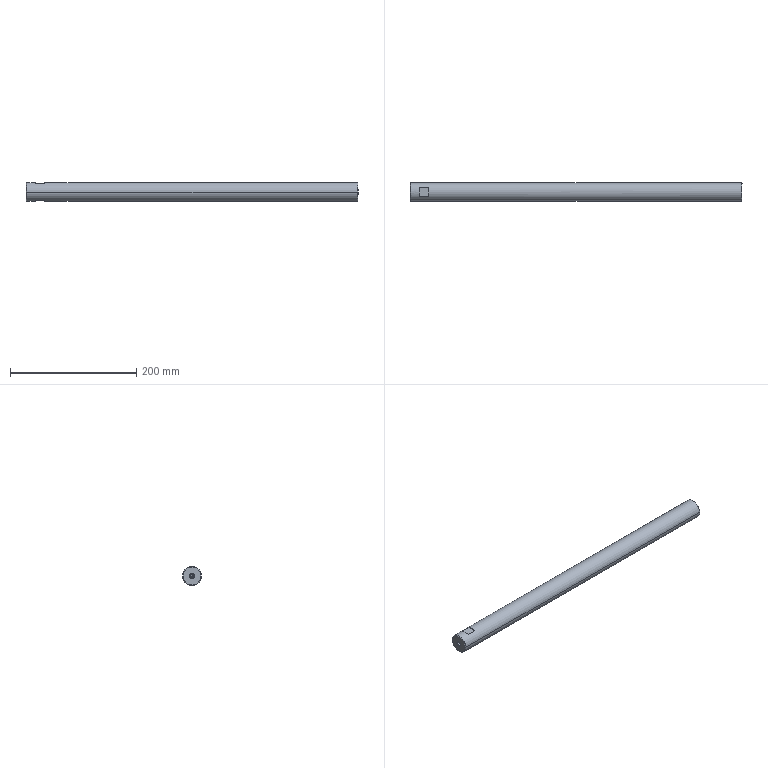Part | SolidWorks | features ICE 1, RevCut 1, Revolution 1 | 1 solid | 20 faces | box 525 x 30 x 30 mm | volume 369974 mm3 | cone 8 | plane 8 | cylinder 4 | commonest cylinder face diameters 6.647 x2 30 x2
STEP:
#1=CARTESIAN_POINT('',(19.519,0.,0.));
#2=VERTEX_POINT('',#1);
#3=CARTESIAN_POINT('',(17.6,-3.324,0.));
#4=VERTEX_POINT('',#3);
#5=CARTESIAN_POINT('',(19.519,0.,0.));
#6=DIRECTION('',(-0.5,-0.866,0.));
#7=VECTOR('',#6,1000.);
#8=LINE('',#5,#7);
#9=EDGE_CURVE('',#2,#4,#8,.T.);
#10=ORIENTED_EDGE('',*,*,#9,.F.);
#11=CARTESIAN_POINT('',(17.6,3.324,0.));
#12=VERTEX_POINT('',#11);
#13=CARTESIAN_POINT('',(19.519,0.,0.));
#14=DIRECTION('',(-0.5,0.866,0.));
#15=VECTOR('',#14,1000.);
#16=LINE('',#13,#15);
#17=EDGE_CURVE('',#2,#12,#16,.T.);
#18=ORIENTED_EDGE('',*,*,#17,.T.);
#19=CARTESIAN_POINT('',(17.6,0.,0.));
#20=DIRECTION('',(-1.,0.,0.));
#21=DIRECTION('',(0.,-1.,0.));
#22=AXIS2_PLACEMENT_3D('',#19,#20,#21);
#23=CIRCLE('',#22,3.324);
#24=EDGE_CURVE('',#12,#4,#23,.T.);
#25=ORIENTED_EDGE('',*,*,#24,.T.);
#26=EDGE_LOOP('',(#10,#18,#25));
#27=FACE_OUTER_BOUND('',#26,.T.);
#28=CARTESIAN_POINT('',(-980.481,0.,0.));
#29=DIRECTION('',(-1.,0.,0.));
#30=DIRECTION('',(0.,-1.,0.));
#31=AXIS2_PLACEMENT_3D('',#28,#29,#30);
#32=CONICAL_SURFACE('',#31,1732.051,1.047);
#33=ADVANCED_FACE('',(#27),#32,.F.);
#34=ORIENTED_EDGE('',*,*,#24,.F.);
#35=CARTESIAN_POINT('',(0.6765,3.324,0.));
#36=VERTEX_POINT('',#35);
#37=CARTESIAN_POINT('',(19.519,3.323,0.));
#38=DIRECTION('',(-1.,0.,0.));
#39=VECTOR('',#38,1000.);
#40=LINE('',#37,#39);
#41=EDGE_CURVE('',#12,#36,#40,.T.);
#42=ORIENTED_EDGE('',*,*,#41,.T.);
#43=CARTESIAN_POINT('',(0.6765,-3.324,0.));
#44=VERTEX_POINT('',#43);
#45=CARTESIAN_POINT('',(0.6765,0.,0.));
#46=DIRECTION('',(-1.,0.,0.));
#47=DIRECTION('',(0.,-1.,0.));
#48=AXIS2_PLACEMENT_3D('',#45,#46,#47);
#49=CIRCLE('',#48,3.324);
#50=EDGE_CURVE('',#36,#44,#49,.T.);
#51=ORIENTED_EDGE('',*,*,#50,.T.);
#52=CARTESIAN_POINT('',(19.519,-3.324,0.));
#53=DIRECTION('',(-1.,0.,0.));
#54=VECTOR('',#53,1000.);
#55=LINE('',#52,#54);
#56=EDGE_CURVE('',#4,#44,#55,.T.);
#57=ORIENTED_EDGE('',*,*,#56,.F.);
#58=EDGE_LOOP('',(#34,#42,#51,#57));
#59=FACE_OUTER_BOUND('',#58,.T.);
#60=CARTESIAN_POINT('',(19.519,0.,0.));
#61=DIRECTION('',(-1.,0.,0.));
#62=DIRECTION('',(0.,-1.,0.));
#63=AXIS2_PLACEMENT_3D('',#60,#61,#62);
#64=CYLINDRICAL_SURFACE('',#63,3.324);
#65=ADVANCED_FACE('',(#59),#64,.F.);
#66=ORIENTED_EDGE('',*,*,#50,.F.);
#67=CARTESIAN_POINT('',(0.,4.,0.));
#68=VERTEX_POINT('',#67);
#69=CARTESIAN_POINT('',(0.6765,3.324,0.));
#70=DIRECTION('',(-0.7071,0.7071,0.));
#71=VECTOR('',#70,1000.);
#72=LINE('',#69,#71);
#73=EDGE_CURVE('',#36,#68,#72,.T.);
#74=ORIENTED_EDGE('',*,*,#73,.T.);
#75=CARTESIAN_POINT('',(0.,-4.,0.));
#76=VERTEX_POINT('',#75);
#77=CARTESIAN_POINT('',(0.,0.,0.));
#78=DIRECTION('',(-1.,0.,0.));
#79=DIRECTION('',(0.,-1.,0.));
#80=AXIS2_PLACEMENT_3D('',#77,#78,#79);
#81=CIRCLE('',#80,4.);
#82=EDGE_CURVE('',#68,#76,#81,.T.);
#83=ORIENTED_EDGE('',*,*,#82,.T.);
#84=CARTESIAN_POINT('',(0.6765,-3.324,0.));
#85=DIRECTION('',(-0.7071,-0.7071,0.));
#86=VECTOR('',#85,1000.);
#87=LINE('',#84,#86);
#88=EDGE_CURVE('',#44,#76,#87,.T.);
#89=ORIENTED_EDGE('',*,*,#88,.F.);
#90=EDGE_LOOP('',(#66,#74,#83,#89));
#91=FACE_OUTER_BOUND('',#90,.T.);
#92=CARTESIAN_POINT('',(0.6765,0.,0.));
#93=DIRECTION('',(-1.,0.,0.));
#94=DIRECTION('',(0.,-1.,0.));
#95=AXIS2_PLACEMENT_3D('',#92,#93,#94);
#96=CONICAL_SURFACE('',#95,3.324,0.7854);
#97=ADVANCED_FACE('',(#91),#96,.F.);
#98=CARTESIAN_POINT('',(525.,-14.,0.));
#99=VERTEX_POINT('',#98);
#100=CARTESIAN_POINT('',(525.,14.,0.));
#101=VERTEX_POINT('',#100);
#102=CARTESIAN_POINT('',(525.,0.,0.));
#103=DIRECTION('',(-1.,0.,0.));
#104=DIRECTION('',(0.,-1.,0.));
#105=AXIS2_PLACEMENT_3D('',#102,#103,#104);
#106=CIRCLE('',#105,14.);
#107=EDGE_CURVE('',#99,#101,#106,.T.);
#108=ORIENTED_EDGE('',*,*,#107,.T.);
#109=CARTESIAN_POINT('',(524.,15.,0.));
#110=VERTEX_POINT('',#109);
#111=CARTESIAN_POINT('',(525.,14.,0.));
#112=DIRECTION('',(-0.7071,0.7071,0.));
#113=VECTOR('',#112,1000.);
#114=LINE('',#111,#113);
#115=EDGE_CURVE('',#101,#110,#114,.T.);
#116=ORIENTED_EDGE('',*,*,#115,.T.);
#117=CARTESIAN_POINT('',(524.,-15.,0.));
#118=VERTEX_POINT('',#117);
#119=CARTESIAN_POINT('',(524.,0.,0.));
#120=DIRECTION('',(-1.,0.,0.));
#121=DIRECTION('',(0.,-1.,0.));
#122=AXIS2_PLACEMENT_3D('',#119,#120,#121);
#123=CIRCLE('',#122,15.);
#124=EDGE_CURVE('',#118,#110,#123,.T.);
#125=ORIENTED_EDGE('',*,*,#124,.F.);
#126=CARTESIAN_POINT('',(525.,-14.,0.));
#127=DIRECTION('',(-0.7071,-0.7071,0.));
#128=VECTOR('',#127,1000.);
#129=LINE('',#126,#128);
#130=EDGE_CURVE('',#99,#118,#129,.T.);
#131=ORIENTED_EDGE('',*,*,#130,.F.);
#132=EDGE_LOOP('',(#108,#116,#125,#131));
#133=FACE_OUTER_BOUND('',#132,.T.);
#134=CARTESIAN_POINT('',(525.,0.,0.));
#135=DIRECTION('',(-1.,0.,0.));
#136=DIRECTION('',(0.,-1.,0.));
#137=AXIS2_PLACEMENT_3D('',#134,#135,#136);
#138=CONICAL_SURFACE('',#137,14.,0.7854);
#139=ADVANCED_FACE('',(#133),#138,.T.);
#140=CARTESIAN_POINT('',(30.,6.538,13.5));
#141=VERTEX_POINT('',#140);
#142=CARTESIAN_POINT('',(30.,-6.538,13.5));
#143=VERTEX_POINT('',#142);
#144=CARTESIAN_POINT('',(30.,0.,0.));
#145=DIRECTION('',(1.,0.,0.));
#146=DIRECTION('',(0.,0.,-1.));
#147=AXIS2_PLACEMENT_3D('',#144,#145,#146);
#148=CIRCLE('',#147,15.);
#149=EDGE_CURVE('',#141,#143,#148,.T.);
#150=ORIENTED_EDGE('',*,*,#149,.T.);
#151=CARTESIAN_POINT('',(15.,-6.538,13.5));
#152=VERTEX_POINT('',#151);
#153=CARTESIAN_POINT('',(525.,-6.538,13.5));
#154=DIRECTION('',(-1.,0.,0.));
#155=VECTOR('',#154,1000.);
#156=LINE('',#153,#155);
#157=EDGE_CURVE('',#143,#152,#156,.T.);
#158=ORIENTED_EDGE('',*,*,#157,.T.);
#159=CARTESIAN_POINT('',(15.,6.538,13.5));
#160=VERTEX_POINT('',#159);
#161=CARTESIAN_POINT('',(15.,0.,0.));
#162=DIRECTION('',(1.,0.,0.));
#163=DIRECTION('',(0.,0.,-1.));
#164=AXIS2_PLACEMENT_3D('',#161,#162,#163);
#165=CIRCLE('',#164,15.);
#166=EDGE_CURVE('',#160,#152,#165,.T.);
#167=ORIENTED_EDGE('',*,*,#166,.F.);
#168=CARTESIAN_POINT('',(525.,6.538,13.5));
#169=DIRECTION('',(1.,0.,0.));
#170=VECTOR('',#169,1000.);
#171=LINE('',#168,#170);
#172=EDGE_CURVE('',#160,#141,#171,.T.);
#173=ORIENTED_EDGE('',*,*,#172,.T.);
#174=EDGE_LOOP('',(#150,#158,#167,#173));
#175=FACE_BOUND('',#174,.T.);
#176=ORIENTED_EDGE('',*,*,#124,.T.);
#177=CARTESIAN_POINT('',(1.,15.,0.));
#178=VERTEX_POINT('',#177);
#179=CARTESIAN_POINT('',(525.,15.,0.));
#180=DIRECTION('',(-1.,0.,0.));
#181=VECTOR('',#180,1000.);
#182=LINE('',#179,#181);
#183=EDGE_CURVE('',#110,#178,#182,.T.);
#184=ORIENTED_EDGE('',*,*,#183,.T.);
#185=CARTESIAN_POINT('',(1.,-15.,0.));
#186=VERTEX_POINT('',#185);
#187=CARTESIAN_POINT('',(1.,0.,0.));
#188=DIRECTION('',(-1.,0.,0.));
#189=DIRECTION('',(0.,-1.,0.));
#190=AXIS2_PLACEMENT_3D('',#187,#188,#189);
#191=CIRCLE('',#190,15.);
#192=EDGE_CURVE('',#186,#178,#191,.T.);
#193=ORIENTED_EDGE('',*,*,#192,.F.);
#194=CARTESIAN_POINT('',(525.,-15.,0.));
#195=DIRECTION('',(-1.,0.,0.));
#196=VECTOR('',#195,1000.);
#197=LINE('',#194,#196);
#198=EDGE_CURVE('',#118,#186,#197,.T.);
#199=ORIENTED_EDGE('',*,*,#198,.F.);
#200=EDGE_LOOP('',(#176,#184,#193,#199));
#201=FACE_OUTER_BOUND('',#200,.T.);
#202=CARTESIAN_POINT('',(525.,0.,0.));
#203=DIRECTION('',(-1.,0.,0.));
#204=DIRECTION('',(0.,-1.,0.));
#205=AXIS2_PLACEMENT_3D('',#202,#203,#204);
#206=CYLINDRICAL_SURFACE('',#205,15.);
#207=ADVANCED_FACE('',(#175,#201),#206,.T.);
#208=CARTESIAN_POINT('',(0.,-14.,0.));
#209=VERTEX_POINT('',#208);
#210=CARTESIAN_POINT('',(0.,14.,0.));
#211=VERTEX_POINT('',#210);
#212=CARTESIAN_POINT('',(0.,0.,0.));
#213=DIRECTION('',(-1.,0.,0.));
#214=DIRECTION('',(0.,-1.,0.));
#215=AXIS2_PLACEMENT_3D('',#212,#213,#214);
#216=CIRCLE('',#215,14.);
#217=EDGE_CURVE('',#209,#211,#216,.T.);
#218=ORIENTED_EDGE('',*,*,#217,.F.);
#219=CARTESIAN_POINT('',(1.,-15.,0.));
#220=DIRECTION('',(0.7071,-0.7071,0.));
#221=VECTOR('',#220,1000.);
#222=LINE('',#219,#221);
#223=EDGE_CURVE('',#209,#186,#222,.T.);
#224=ORIENTED_EDGE('',*,*,#223,.T.);
#225=ORIENTED_EDGE('',*,*,#192,.T.);
#226=CARTESIAN_POINT('',(1.,15.,0.));
#227=DIRECTION('',(0.7071,0.7071,0.));
#228=VECTOR('',#227,1000.);
#229=LINE('',#226,#228);
#230=EDGE_CURVE('',#211,#178,#229,.T.);
#231=ORIENTED_EDGE('',*,*,#230,.F.);
#232=EDGE_LOOP('',(#218,#224,#225,#231));
#233=FACE_OUTER_BOUND('',#232,.T.);
#234=CARTESIAN_POINT('',(1.,0.,0.));
#235=DIRECTION('',(1.,0.,0.));
#236=DIRECTION('',(0.,1.,0.));
#237=AXIS2_PLACEMENT_3D('',#234,#235,#236);
#238=CONICAL_SURFACE('',#237,15.,0.7854);
#239=ADVANCED_FACE('',(#233),#238,.T.);
#240=CARTESIAN_POINT('',(0.,0.,0.));
#241=DIRECTION('',(-1.,0.,0.));
#242=DIRECTION('',(0.,-1.,0.));
#243=AXIS2_PLACEMENT_3D('',#240,#241,#242);
#244=CIRCLE('',#243,14.);
#245=EDGE_CURVE('',#211,#209,#244,.T.);
#246=ORIENTED_EDGE('',*,*,#245,.T.);
#247=ORIENTED_EDGE('',*,*,#217,.T.);
#248=EDGE_LOOP('',(#246,#247));
#249=FACE_OUTER_BOUND('',#248,.T.);
#250=CARTESIAN_POINT('',(0.,0.,0.));
#251=DIRECTION('',(-1.,0.,0.));
#252=DIRECTION('',(0.,-1.,0.));
#253=AXIS2_PLACEMENT_3D('',#250,#251,#252);
#254=CIRCLE('',#253,4.);
#255=EDGE_CURVE('',#76,#68,#254,.T.);
#256=ORIENTED_EDGE('',*,*,#255,.F.);
#257=ORIENTED_EDGE('',*,*,#82,.F.);
#258=EDGE_LOOP('',(#256,#257));
#259=FACE_BOUND('',#258,.T.);
#260=CARTESIAN_POINT('',(0.,0.,0.));
#261=DIRECTION('',(1.,0.,0.));
#262=DIRECTION('',(0.,1.,0.));
#263=AXIS2_PLACEMENT_3D('',#260,#261,#262);
#264=PLANE('',#263);
#265=ADVANCED_FACE('',(#249,#259),#264,.F.);
#266=ORIENTED_EDGE('',*,*,#223,.F.);
#267=ORIENTED_EDGE('',*,*,#245,.F.);
#268=ORIENTED_EDGE('',*,*,#230,.T.);
#269=CARTESIAN_POINT('',(1.,0.,0.));
#270=DIRECTION('',(-1.,0.,0.));
#271=DIRECTION('',(0.,-1.,0.));
#272=AXIS2_PLACEMENT_3D('',#269,#270,#271);
#273=CIRCLE('',#272,15.);
#274=EDGE_CURVE('',#178,#186,#273,.T.);
#275=ORIENTED_EDGE('',*,*,#274,.T.);
#276=EDGE_LOOP('',(#266,#267,#268,#275));
#277=FACE_OUTER_BOUND('',#276,.T.);
#278=CARTESIAN_POINT('',(1.,0.,0.));
#279=DIRECTION('',(1.,0.,0.));
#280=DIRECTION('',(0.,1.,0.));
#281=AXIS2_PLACEMENT_3D('',#278,#279,#280);
#282=CONICAL_SURFACE('',#281,15.,0.7854);
#283=ADVANCED_FACE('',(#277),#282,.T.);
#284=ORIENTED_EDGE('',*,*,#183,.F.);
#285=CARTESIAN_POINT('',(524.,0.,0.));
#286=DIRECTION('',(-1.,0.,0.));
#287=DIRECTION('',(0.,-1.,0.));
#288=AXIS2_PLACEMENT_3D('',#285,#286,#287);
#289=CIRCLE('',#288,15.);
#290=EDGE_CURVE('',#110,#118,#289,.T.);
#291=ORIENTED_EDGE('',*,*,#290,.T.);
#292=ORIENTED_EDGE('',*,*,#198,.T.);
#293=ORIENTED_EDGE('',*,*,#274,.F.);
#294=EDGE_LOOP('',(#284,#291,#292,#293));
#295=FACE_OUTER_BOUND('',#294,.T.);
#296=CARTESIAN_POINT('',(30.,-6.538,-13.5));
#297=VERTEX_POINT('',#296);
#298=CARTESIAN_POINT('',(30.,6.538,-13.5));
#299=VERTEX_POINT('',#298);
#300=CARTESIAN_POINT('',(30.,0.,0.));
#301=DIRECTION('',(1.,0.,0.));
#302=DIRECTION('',(0.,0.,-1.));
#303=AXIS2_PLACEMENT_3D('',#300,#301,#302);
#304=CIRCLE('',#303,15.);
#305=EDGE_CURVE('',#297,#299,#304,.T.);
#306=ORIENTED_EDGE('',*,*,#305,.T.);
#307=CARTESIAN_POINT('',(15.,6.538,-13.5));
#308=VERTEX_POINT('',#307);
#309=CARTESIAN_POINT('',(525.,6.538,-13.5));
#310=DIRECTION('',(-1.,0.,0.));
#311=VECTOR('',#310,1000.);
#312=LINE('',#309,#311);
#313=EDGE_CURVE('',#299,#308,#312,.T.);
#314=ORIENTED_EDGE('',*,*,#313,.T.);
#315=CARTESIAN_POINT('',(15.,-6.538,-13.5));
#316=VERTEX_POINT('',#315);
#317=CARTESIAN_POINT('',(15.,0.,0.));
#318=DIRECTION('',(1.,0.,0.));
#319=DIRECTION('',(0.,0.,-1.));
#320=AXIS2_PLACEMENT_3D('',#317,#318,#319);
#321=CIRCLE('',#320,15.);
#322=EDGE_CURVE('',#316,#308,#321,.T.);
#323=ORIENTED_EDGE('',*,*,#322,.F.);
#324=CARTESIAN_POINT('',(525.,-6.538,-13.5));
#325=DIRECTION('',(1.,0.,0.));
#326=VECTOR('',#325,1000.);
#327=LINE('',#324,#326);
#328=EDGE_CURVE('',#316,#297,#327,.T.);
#329=ORIENTED_EDGE('',*,*,#328,.T.);
#330=EDGE_LOOP('',(#306,#314,#323,#329));
#331=FACE_BOUND('',#330,.T.);
#332=CARTESIAN_POINT('',(525.,0.,0.));
#333=DIRECTION('',(-1.,0.,0.));
#334=DIRECTION('',(0.,-1.,0.));
#335=AXIS2_PLACEMENT_3D('',#332,#333,#334);
#336=CYLINDRICAL_SURFACE('',#335,15.);
#337=ADVANCED_FACE('',(#295,#331),#336,.T.);
#338=ORIENTED_EDGE('',*,*,#115,.F.);
#339=CARTESIAN_POINT('',(525.,0.,0.));
#340=DIRECTION('',(-1.,0.,0.));
#341=DIRECTION('',(0.,-1.,0.));
#342=AXIS2_PLACEMENT_3D('',#339,#340,#341);
#343=CIRCLE('',#342,14.);
#344=EDGE_CURVE('',#101,#99,#343,.T.);
#345=ORIENTED_EDGE('',*,*,#344,.T.);
#346=ORIENTED_EDGE('',*,*,#130,.T.);
#347=ORIENTED_EDGE('',*,*,#290,.F.);
#348=EDGE_LOOP('',(#338,#345,#346,#347));
#349=FACE_OUTER_BOUND('',#348,.T.);
#350=CARTESIAN_POINT('',(525.,0.,0.));
#351=DIRECTION('',(-1.,0.,0.));
#352=DIRECTION('',(0.,-1.,0.));
#353=AXIS2_PLACEMENT_3D('',#350,#351,#352);
#354=CONICAL_SURFACE('',#353,14.,0.7854);
#355=ADVANCED_FACE('',(#349),#354,.T.);
#356=ORIENTED_EDGE('',*,*,#107,.F.);
#357=ORIENTED_EDGE('',*,*,#344,.F.);
#358=EDGE_LOOP('',(#356,#357));
#359=FACE_OUTER_BOUND('',#358,.T.);
#360=CARTESIAN_POINT('',(525.,14.,0.));
#361=DIRECTION('',(-1.,0.,0.));
#362=DIRECTION('',(0.,-1.,0.));
#363=AXIS2_PLACEMENT_3D('',#360,#361,#362);
#364=PLANE('',#363);
#365=ADVANCED_FACE('',(#359),#364,.F.);
#366=ORIENTED_EDGE('',*,*,#73,.F.);
#367=CARTESIAN_POINT('',(0.6765,0.,0.));
#368=DIRECTION('',(-1.,0.,0.));
#369=DIRECTION('',(0.,-1.,0.));
#370=AXIS2_PLACEMENT_3D('',#367,#368,#369);
#371=CIRCLE('',#370,3.324);
#372=EDGE_CURVE('',#44,#36,#371,.T.);
#373=ORIENTED_EDGE('',*,*,#372,.F.);
#374=ORIENTED_EDGE('',*,*,#88,.T.);
#375=ORIENTED_EDGE('',*,*,#255,.T.);
#376=EDGE_LOOP('',(#366,#373,#374,#375));
#377=FACE_OUTER_BOUND('',#376,.T.);
#378=CARTESIAN_POINT('',(0.6765,0.,0.));
#379=DIRECTION('',(-1.,0.,0.));
#380=DIRECTION('',(0.,-1.,0.));
#381=AXIS2_PLACEMENT_3D('',#378,#379,#380);
#382=CONICAL_SURFACE('',#381,3.324,0.7854);
#383=ADVANCED_FACE('',(#377),#382,.F.);
#384=ORIENTED_EDGE('',*,*,#41,.F.);
#385=CARTESIAN_POINT('',(17.6,0.,0.));
#386=DIRECTION('',(-1.,0.,0.));
#387=DIRECTION('',(0.,-1.,0.));
#388=AXIS2_PLACEMENT_3D('',#385,#386,#387);
#389=CIRCLE('',#388,3.324);
#390=EDGE_CURVE('',#4,#12,#389,.T.);
#391=ORIENTED_EDGE('',*,*,#390,.F.);
#392=ORIENTED_EDGE('',*,*,#56,.T.);
#393=ORIENTED_EDGE('',*,*,#372,.T.);
#394=EDGE_LOOP('',(#384,#391,#392,#393));
#395=FACE_OUTER_BOUND('',#394,.T.);
#396=CARTESIAN_POINT('',(19.519,0.,0.));
#397=DIRECTION('',(-1.,0.,0.));
#398=DIRECTION('',(0.,-1.,0.));
#399=AXIS2_PLACEMENT_3D('',#396,#397,#398);
#400=CYLINDRICAL_SURFACE('',#399,3.324);
#401=ADVANCED_FACE('',(#395),#400,.F.);
#402=ORIENTED_EDGE('',*,*,#17,.F.);
#403=ORIENTED_EDGE('',*,*,#9,.T.);
#404=ORIENTED_EDGE('',*,*,#390,.T.);
#405=EDGE_LOOP('',(#402,#403,#404));
#406=FACE_OUTER_BOUND('',#405,.T.);
#407=CARTESIAN_POINT('',(-980.481,0.,0.));
#408=DIRECTION('',(-1.,0.,0.));
#409=DIRECTION('',(0.,-1.,0.));
#410=AXIS2_PLACEMENT_3D('',#407,#408,#409);
#411=CONICAL_SURFACE('',#410,1732.051,1.047);
#412=ADVANCED_FACE('',(#406),#411,.F.);
#413=CARTESIAN_POINT('',(30.,-30.,-13.5));
#414=DIRECTION('',(0.,1.,0.));
#415=VECTOR('',#414,1000.);
#416=LINE('',#413,#415);
#417=EDGE_CURVE('',#297,#299,#416,.T.);
#418=ORIENTED_EDGE('',*,*,#417,.F.);
#419=ORIENTED_EDGE('',*,*,#328,.F.);
#420=CARTESIAN_POINT('',(15.,-30.,-13.5));
#421=DIRECTION('',(0.,1.,0.));
#422=VECTOR('',#421,1000.);
#423=LINE('',#420,#422);
#424=EDGE_CURVE('',#316,#308,#423,.T.);
#425=ORIENTED_EDGE('',*,*,#424,.T.);
#426=ORIENTED_EDGE('',*,*,#313,.F.);
#427=EDGE_LOOP('',(#418,#419,#425,#426));
#428=FACE_OUTER_BOUND('',#427,.T.);
#429=CARTESIAN_POINT('',(30.,-30.,-13.5));
#430=DIRECTION('',(0.,0.,1.));
#431=DIRECTION('',(1.,0.,0.));
#432=AXIS2_PLACEMENT_3D('',#429,#430,#431);
#433=PLANE('',#432);
#434=ADVANCED_FACE('',(#428),#433,.F.);
#435=ORIENTED_EDGE('',*,*,#322,.T.);
#436=ORIENTED_EDGE('',*,*,#424,.F.);
#437=EDGE_LOOP('',(#435,#436));
#438=FACE_OUTER_BOUND('',#437,.T.);
#439=CARTESIAN_POINT('',(15.,0.,0.));
#440=DIRECTION('',(1.,0.,0.));
#441=DIRECTION('',(0.,0.,-1.));
#442=AXIS2_PLACEMENT_3D('',#439,#440,#441);
#443=PLANE('',#442);
#444=ADVANCED_FACE('',(#438),#443,.T.);
#445=ORIENTED_EDGE('',*,*,#417,.T.);
#446=ORIENTED_EDGE('',*,*,#305,.F.);
#447=EDGE_LOOP('',(#445,#446));
#448=FACE_OUTER_BOUND('',#447,.T.);
#449=CARTESIAN_POINT('',(30.,0.,0.));
#450=DIRECTION('',(1.,0.,0.));
#451=DIRECTION('',(0.,0.,-1.));
#452=AXIS2_PLACEMENT_3D('',#449,#450,#451);
#453=PLANE('',#452);
#454=ADVANCED_FACE('',(#448),#453,.F.);
#455=CARTESIAN_POINT('',(30.,30.,13.5));
#456=DIRECTION('',(0.,-1.,0.));
#457=VECTOR('',#456,1000.);
#458=LINE('',#455,#457);
#459=EDGE_CURVE('',#141,#143,#458,.T.);
#460=ORIENTED_EDGE('',*,*,#459,.T.);
#461=ORIENTED_EDGE('',*,*,#149,.F.);
#462=EDGE_LOOP('',(#460,#461));
#463=FACE_OUTER_BOUND('',#462,.T.);
#464=CARTESIAN_POINT('',(30.,0.,0.));
#465=DIRECTION('',(1.,0.,0.));
#466=DIRECTION('',(0.,0.,-1.));
#467=AXIS2_PLACEMENT_3D('',#464,#465,#466);
#468=PLANE('',#467);
#469=ADVANCED_FACE('',(#463),#468,.F.);
#470=ORIENTED_EDGE('',*,*,#166,.T.);
#471=CARTESIAN_POINT('',(15.,30.,13.5));
#472=DIRECTION('',(0.,-1.,0.));
#473=VECTOR('',#472,1000.);
#474=LINE('',#471,#473);
#475=EDGE_CURVE('',#160,#152,#474,.T.);
#476=ORIENTED_EDGE('',*,*,#475,.F.);
#477=EDGE_LOOP('',(#470,#476));
#478=FACE_OUTER_BOUND('',#477,.T.);
#479=CARTESIAN_POINT('',(15.,0.,0.));
#480=DIRECTION('',(1.,0.,0.));
#481=DIRECTION('',(0.,0.,-1.));
#482=AXIS2_PLACEMENT_3D('',#479,#480,#481);
#483=PLANE('',#482);
#484=ADVANCED_FACE('',(#478),#483,.T.);
#485=ORIENTED_EDGE('',*,*,#459,.F.);
#486=ORIENTED_EDGE('',*,*,#172,.F.);
#487=ORIENTED_EDGE('',*,*,#475,.T.);
#488=ORIENTED_EDGE('',*,*,#157,.F.);
#489=EDGE_LOOP('',(#485,#486,#487,#488));
#490=FACE_OUTER_BOUND('',#489,.T.);
#491=CARTESIAN_POINT('',(30.,30.,13.5));
#492=DIRECTION('',(0.,0.,-1.));
#493=DIRECTION('',(-1.,0.,0.));
#494=AXIS2_PLACEMENT_3D('',#491,#492,#493);
#495=PLANE('',#494);
#496=ADVANCED_FACE('',(#490),#495,.F.);
#497=CLOSED_SHELL('',(#33,#65,#97,#139,#207,#239,#265,#283,#337,#355,#365,#383,#401,#412,#434,#444,#454,#469,#484,#496));
#498=MANIFOLD_SOLID_BREP('',#497);
#499=CARTESIAN_POINT('',(0.,0.,0.));
#500=DIRECTION('',(0.,0.,1.));
#501=DIRECTION('',(1.,0.,0.));
#502=AXIS2_PLACEMENT_3D('',#499,#500,#501);
#503=(LENGTH_UNIT()NAMED_UNIT(*)SI_UNIT(.MILLI.,.METRE.));
#504=UNCERTAINTY_MEASURE_WITH_UNIT(LENGTH_MEASURE(0.00001),#503,'','');
#505=(NAMED_UNIT(*)PLANE_ANGLE_UNIT()SI_UNIT($,.RADIAN.));
#506=(NAMED_UNIT(*)SI_UNIT($,.STERADIAN.)SOLID_ANGLE_UNIT());
#507=(GEOMETRIC_REPRESENTATION_CONTEXT(3)GLOBAL_UNCERTAINTY_ASSIGNED_CONTEXT((#504))GLOBAL_UNIT_ASSIGNED_CONTEXT((#503,#505,#506))REPRESENTATION_CONTEXT('',''));
#508=ADVANCED_BREP_SHAPE_REPRESENTATION('',(#498,#502),#507);